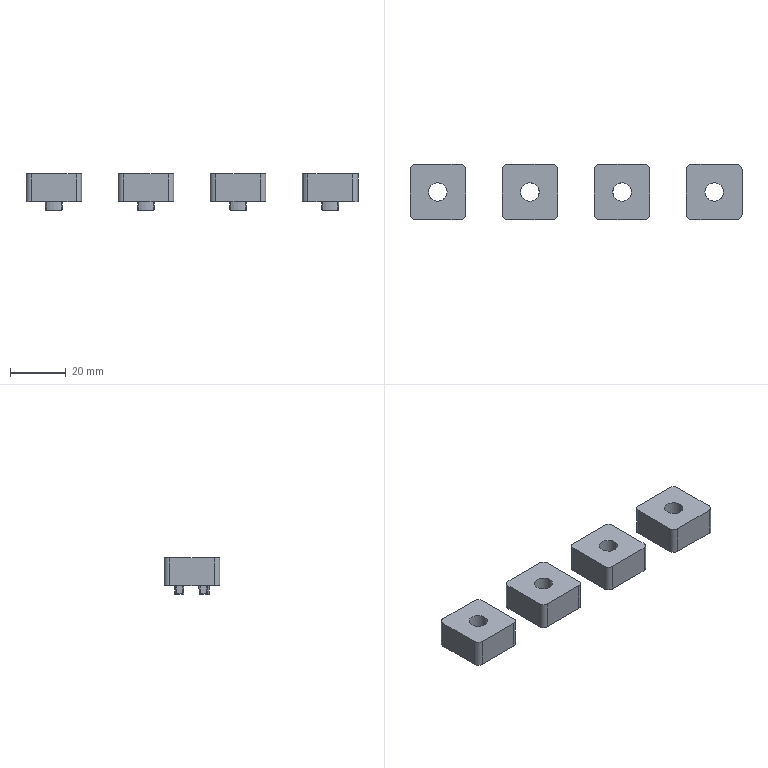NC program | NX | posted with a generic post | part box 118.91 x 19.91 x 13 mm
Lines 1 to 18 of 17620:
N10 G17 G21 G94 G90
(FLOOR_WALL , TOOL : D80)
N12 T19 M6
N14 G54
N16 G17 G0 G90 X104.455 Y0. S6500 M3
N18 G43 Z30. H19
N20 Z3.
N22 G94 G1 Z0. F1500.
N24 X101.455
N26 X-101.455
N28 X-104.455
N30 Z3.
N32 G0 Z30.
N34 M5